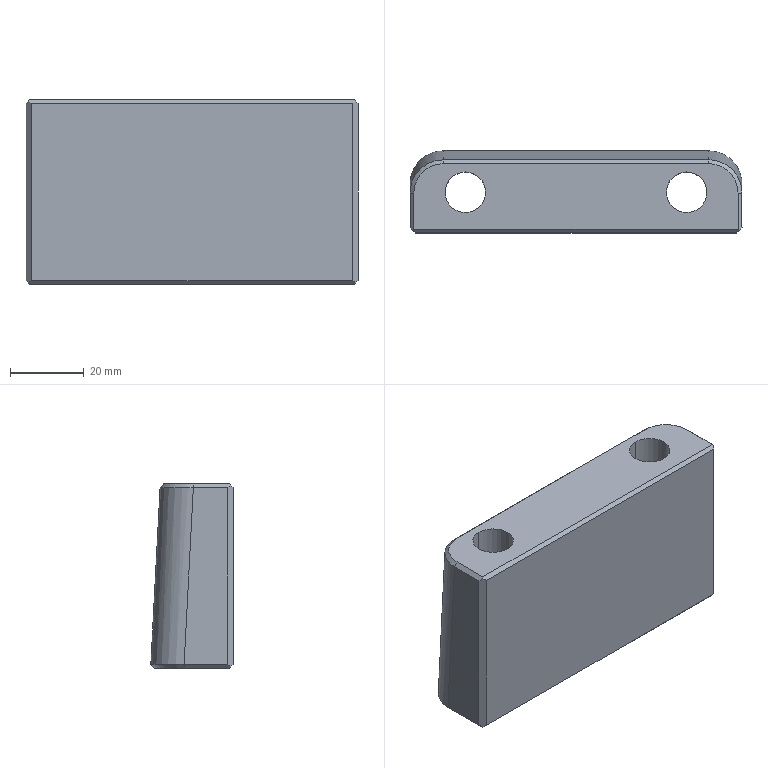Part | Creo | 1 solid | 39 faces | box 90 x 22.317 x 50 mm | volume 78698 mm3 | plane 19 | cylinder 14 | spline 4 | cone 2 | commonest cylinder face diameters 18 x6 11 x4 7 x2 8 x2
STEP:
#1=CARTESIAN_POINT('',(-25.,211.995,61.));
#2=VERTEX_POINT('',#1);
#3=CARTESIAN_POINT('',(-25.,229.995,61.));
#4=VERTEX_POINT('',#3);
#5=CARTESIAN_POINT('',(-25.,220.995,61.));
#6=DIRECTION('',(0.,0.,-1.));
#7=DIRECTION('',(0.000000059,-1.,0.));
#8=AXIS2_PLACEMENT_3D('',#5,#6,#7);
#9=CIRCLE('',#8,9.);
#10=EDGE_CURVE('',#2,#4,#9,.T.);
#11=ORIENTED_EDGE('',*,*,#10,.T.);
#12=CARTESIAN_POINT('',(-25.,229.995,50.));
#13=VERTEX_POINT('',#12);
#14=CARTESIAN_POINT('',(-25.,229.995,50.));
#15=DIRECTION('',(0.,0.,1.));
#16=VECTOR('',#15,11.);
#17=LINE('',#14,#16);
#18=EDGE_CURVE('',#13,#4,#17,.T.);
#19=ORIENTED_EDGE('',*,*,#18,.F.);
#20=CARTESIAN_POINT('',(-34.,220.995,50.));
#21=VERTEX_POINT('',#20);
#22=CARTESIAN_POINT('',(-25.,220.995,50.));
#23=DIRECTION('',(0.,0.,1.));
#24=DIRECTION('',(-0.000000059,1.,0.));
#25=AXIS2_PLACEMENT_3D('',#22,#23,#24);
#26=CIRCLE('',#25,9.);
#27=EDGE_CURVE('',#13,#21,#26,.T.);
#28=ORIENTED_EDGE('',*,*,#27,.T.);
#29=CARTESIAN_POINT('',(-25.,211.995,50.));
#30=VERTEX_POINT('',#29);
#31=CARTESIAN_POINT('',(-25.,220.995,50.));
#32=DIRECTION('',(0.,0.,1.));
#33=DIRECTION('',(-1.,0.,0.));
#34=AXIS2_PLACEMENT_3D('',#31,#32,#33);
#35=CIRCLE('',#34,9.);
#36=EDGE_CURVE('',#21,#30,#35,.T.);
#37=ORIENTED_EDGE('',*,*,#36,.T.);
#38=CARTESIAN_POINT('',(-25.,211.995,50.));
#39=DIRECTION('',(0.,0.,1.));
#40=VECTOR('',#39,11.);
#41=LINE('',#38,#40);
#42=EDGE_CURVE('',#30,#2,#41,.T.);
#43=ORIENTED_EDGE('',*,*,#42,.T.);
#44=EDGE_LOOP('',(#11,#19,#28,#37,#43));
#45=FACE_OUTER_BOUND('',#44,.F.);
#46=CARTESIAN_POINT('',(-25.,220.995,63.45));
#47=DIRECTION('',(0.,0.,1.));
#48=DIRECTION('',(-0.000000059,1.,0.));
#49=AXIS2_PLACEMENT_3D('',#46,#47,#48);
#50=CYLINDRICAL_SURFACE('',#49,9.);
#51=ADVANCED_FACE('',(#45),#50,.F.);
#52=CARTESIAN_POINT('',(-16.,220.995,61.));
#53=VERTEX_POINT('',#52);
#54=CARTESIAN_POINT('',(-25.,220.995,61.));
#55=DIRECTION('',(0.,0.,-1.));
#56=DIRECTION('',(1.,0.,0.));
#57=AXIS2_PLACEMENT_3D('',#54,#55,#56);
#58=CIRCLE('',#57,9.);
#59=EDGE_CURVE('',#53,#2,#58,.T.);
#60=ORIENTED_EDGE('',*,*,#59,.F.);
#61=CARTESIAN_POINT('',(-25.,220.995,61.));
#62=DIRECTION('',(0.,0.,-1.));
#63=DIRECTION('',(-0.000000059,1.,0.));
#64=AXIS2_PLACEMENT_3D('',#61,#62,#63);
#65=CIRCLE('',#64,9.);
#66=EDGE_CURVE('',#4,#53,#65,.T.);
#67=ORIENTED_EDGE('',*,*,#66,.F.);
#68=ORIENTED_EDGE('',*,*,#10,.F.);
#69=EDGE_LOOP('',(#60,#67,#68));
#70=FACE_OUTER_BOUND('',#69,.F.);
#71=CARTESIAN_POINT('',(-19.5,220.995,61.));
#72=VERTEX_POINT('',#71);
#73=CARTESIAN_POINT('',(-25.,226.495,61.));
#74=VERTEX_POINT('',#73);
#75=CARTESIAN_POINT('',(-25.,220.995,61.));
#76=DIRECTION('',(0.,0.,1.));
#77=DIRECTION('',(1.,0.,0.));
#78=AXIS2_PLACEMENT_3D('',#75,#76,#77);
#79=CIRCLE('',#78,5.5);
#80=EDGE_CURVE('',#72,#74,#79,.T.);
#81=ORIENTED_EDGE('',*,*,#80,.F.);
#82=CARTESIAN_POINT('',(-25.,215.495,61.));
#83=VERTEX_POINT('',#82);
#84=CARTESIAN_POINT('',(-25.,220.995,61.));
#85=DIRECTION('',(0.,0.,1.));
#86=DIRECTION('',(0.000000059,-1.,0.));
#87=AXIS2_PLACEMENT_3D('',#84,#85,#86);
#88=CIRCLE('',#87,5.5);
#89=EDGE_CURVE('',#83,#72,#88,.T.);
#90=ORIENTED_EDGE('',*,*,#89,.F.);
#91=CARTESIAN_POINT('',(-25.,220.995,61.));
#92=DIRECTION('',(0.,0.,1.));
#93=DIRECTION('',(-0.000000059,1.,0.));
#94=AXIS2_PLACEMENT_3D('',#91,#92,#93);
#95=CIRCLE('',#94,5.5);
#96=EDGE_CURVE('',#74,#83,#95,.T.);
#97=ORIENTED_EDGE('',*,*,#96,.F.);
#98=EDGE_LOOP('',(#81,#90,#97));
#99=FACE_BOUND('',#98,.F.);
#100=CARTESIAN_POINT('',(-25.,220.995,61.));
#101=DIRECTION('',(0.,0.,1.));
#102=DIRECTION('',(-0.000000059,1.,0.));
#103=AXIS2_PLACEMENT_3D('',#100,#101,#102);
#104=PLANE('',#103);
#105=ADVANCED_FACE('',(#70,#99),#104,.F.);
#106=CARTESIAN_POINT('',(-25.,226.495,100.));
#107=VERTEX_POINT('',#106);
#108=CARTESIAN_POINT('',(-25.,215.495,100.));
#109=VERTEX_POINT('',#108);
#110=CARTESIAN_POINT('',(-25.,220.995,100.));
#111=DIRECTION('',(0.,0.,-1.));
#112=DIRECTION('',(-0.000000059,1.,0.));
#113=AXIS2_PLACEMENT_3D('',#110,#111,#112);
#114=CIRCLE('',#113,5.5);
#115=EDGE_CURVE('',#107,#109,#114,.T.);
#116=ORIENTED_EDGE('',*,*,#115,.T.);
#117=CARTESIAN_POINT('',(-25.,215.495,100.));
#118=DIRECTION('',(0.,0.,-1.));
#119=VECTOR('',#118,39.);
#120=LINE('',#117,#119);
#121=EDGE_CURVE('',#109,#83,#120,.T.);
#122=ORIENTED_EDGE('',*,*,#121,.T.);
#123=ORIENTED_EDGE('',*,*,#89,.T.);
#124=ORIENTED_EDGE('',*,*,#80,.T.);
#125=CARTESIAN_POINT('',(-25.,226.495,100.));
#126=DIRECTION('',(0.,0.,-1.));
#127=VECTOR('',#126,39.);
#128=LINE('',#125,#127);
#129=EDGE_CURVE('',#107,#74,#128,.T.);
#130=ORIENTED_EDGE('',*,*,#129,.F.);
#131=EDGE_LOOP('',(#116,#122,#123,#124,#130));
#132=FACE_OUTER_BOUND('',#131,.F.);
#133=CARTESIAN_POINT('',(-25.,220.995,75.));
#134=DIRECTION('',(0.,0.,-1.));
#135=DIRECTION('',(-0.000000059,1.,0.));
#136=AXIS2_PLACEMENT_3D('',#133,#134,#135);
#137=CYLINDRICAL_SURFACE('',#136,5.5);
#138=ADVANCED_FACE('',(#132),#137,.F.);
#139=CARTESIAN_POINT('',(-91.,228.755,100.));
#140=VERTEX_POINT('',#139);
#141=CARTESIAN_POINT('',(-98.946,220.797,100.));
#142=VERTEX_POINT('',#141);
#143=CARTESIAN_POINT('',(-93.083,228.763,100.));
#144=CARTESIAN_POINT('',(-97.219,227.025,100.));
#145=CARTESIAN_POINT('',(-98.955,222.883,100.));
#146=B_SPLINE_CURVE_WITH_KNOTS('',3,(#139,#143,#144,#145,#141),.UNSPECIFIED.,.F.,.F.,(4,1,4),(0.,0.5,1.),.UNSPECIFIED.);
#147=EDGE_CURVE('',#140,#142,#146,.T.);
#148=ORIENTED_EDGE('',*,*,#147,.F.);
#149=CARTESIAN_POINT('',(-19.,228.755,100.));
#150=VERTEX_POINT('',#149);
#151=CARTESIAN_POINT('',(-91.,228.755,100.));
#152=DIRECTION('',(1.,0.000000059,0.));
#153=VECTOR('',#152,72.);
#154=LINE('',#151,#153);
#155=EDGE_CURVE('',#140,#150,#154,.T.);
#156=ORIENTED_EDGE('',*,*,#155,.T.);
#157=CARTESIAN_POINT('',(-11.054,220.797,100.));
#158=VERTEX_POINT('',#157);
#159=CARTESIAN_POINT('',(-11.054,220.797,100.));
#160=CARTESIAN_POINT('',(-11.045,222.883,100.));
#161=CARTESIAN_POINT('',(-12.781,227.025,100.));
#162=CARTESIAN_POINT('',(-16.917,228.763,100.));
#163=B_SPLINE_CURVE_WITH_KNOTS('',3,(#159,#160,#161,#162,#149),.UNSPECIFIED.,.F.,.F.,(4,1,4),(0.,0.5,1.),.UNSPECIFIED.);
#164=EDGE_CURVE('',#158,#150,#163,.T.);
#165=ORIENTED_EDGE('',*,*,#164,.F.);
#166=CARTESIAN_POINT('',(-11.054,210.944,100.));
#167=VERTEX_POINT('',#166);
#168=CARTESIAN_POINT('',(-11.054,220.797,100.));
#169=DIRECTION('',(0.000000059,-1.,0.));
#170=VECTOR('',#169,9.853);
#171=LINE('',#168,#170);
#172=EDGE_CURVE('',#158,#167,#171,.T.);
#173=ORIENTED_EDGE('',*,*,#172,.T.);
#174=CARTESIAN_POINT('',(-98.946,210.944,100.));
#175=VERTEX_POINT('',#174);
#176=CARTESIAN_POINT('',(-11.054,210.944,100.));
#177=DIRECTION('',(-1.,-0.000000059,0.));
#178=VECTOR('',#177,87.892);
#179=LINE('',#176,#178);
#180=EDGE_CURVE('',#167,#175,#179,.T.);
#181=ORIENTED_EDGE('',*,*,#180,.T.);
#182=CARTESIAN_POINT('',(-98.946,210.944,100.));
#183=DIRECTION('',(-0.000000059,1.,0.));
#184=VECTOR('',#183,9.853);
#185=LINE('',#182,#184);
#186=EDGE_CURVE('',#175,#142,#185,.T.);
#187=ORIENTED_EDGE('',*,*,#186,.T.);
#188=EDGE_LOOP('',(#148,#156,#165,#173,#181,#187));
#189=FACE_OUTER_BOUND('',#188,.F.);
#190=ORIENTED_EDGE('',*,*,#115,.F.);
#191=CARTESIAN_POINT('',(-25.,220.995,100.));
#192=DIRECTION('',(0.,0.,-1.));
#193=DIRECTION('',(0.000000059,-1.,0.));
#194=AXIS2_PLACEMENT_3D('',#191,#192,#193);
#195=CIRCLE('',#194,5.5);
#196=EDGE_CURVE('',#109,#107,#195,.T.);
#197=ORIENTED_EDGE('',*,*,#196,.F.);
#198=EDGE_LOOP('',(#190,#197));
#199=FACE_BOUND('',#198,.F.);
#200=CARTESIAN_POINT('',(-85.,226.495,100.));
#201=VERTEX_POINT('',#200);
#202=CARTESIAN_POINT('',(-85.,215.495,100.));
#203=VERTEX_POINT('',#202);
#204=CARTESIAN_POINT('',(-85.,220.995,100.));
#205=DIRECTION('',(0.,0.,-1.));
#206=DIRECTION('',(-0.000000059,1.,0.));
#207=AXIS2_PLACEMENT_3D('',#204,#205,#206);
#208=CIRCLE('',#207,5.5);
#209=EDGE_CURVE('',#201,#203,#208,.T.);
#210=ORIENTED_EDGE('',*,*,#209,.F.);
#211=CARTESIAN_POINT('',(-85.,220.995,100.));
#212=DIRECTION('',(0.,0.,-1.));
#213=DIRECTION('',(0.000000059,-1.,0.));
#214=AXIS2_PLACEMENT_3D('',#211,#212,#213);
#215=CIRCLE('',#214,5.5);
#216=EDGE_CURVE('',#203,#201,#215,.T.);
#217=ORIENTED_EDGE('',*,*,#216,.F.);
#218=EDGE_LOOP('',(#210,#217));
#219=FACE_BOUND('',#218,.F.);
#220=CARTESIAN_POINT('',(-10.,209.995,100.));
#221=DIRECTION('',(0.,0.,1.));
#222=DIRECTION('',(-0.000000059,1.,0.));
#223=AXIS2_PLACEMENT_3D('',#220,#221,#222);
#224=PLANE('',#223);
#225=ADVANCED_FACE('',(#189,#199,#219),#224,.T.);
#226=CARTESIAN_POINT('',(-91.,229.807,99.001));
#227=VERTEX_POINT('',#226);
#228=CARTESIAN_POINT('',(-91.,228.755,100.));
#229=DIRECTION('',(0.000000048,0.7254,-0.6884));
#230=VECTOR('',#229,1.451);
#231=LINE('',#228,#230);
#232=EDGE_CURVE('',#140,#227,#231,.T.);
#233=ORIENTED_EDGE('',*,*,#232,.F.);
#234=ORIENTED_EDGE('',*,*,#147,.T.);
#235=CARTESIAN_POINT('',(-100.,220.797,98.946));
#236=VERTEX_POINT('',#235);
#237=CARTESIAN_POINT('',(-100.,220.797,98.946));
#238=DIRECTION('',(0.7071,0.000000042,0.7071));
#239=VECTOR('',#238,1.49);
#240=LINE('',#237,#239);
#241=EDGE_CURVE('',#236,#142,#240,.T.);
#242=ORIENTED_EDGE('',*,*,#241,.F.);
#243=CARTESIAN_POINT('',(-91.,229.807,99.001));
#244=CARTESIAN_POINT('',(-91.278,229.807,99.003));
#245=CARTESIAN_POINT('',(-91.835,229.781,99.003));
#246=CARTESIAN_POINT('',(-92.662,229.665,99.));
#247=CARTESIAN_POINT('',(-93.474,229.473,98.996));
#248=CARTESIAN_POINT('',(-94.266,229.207,98.992));
#249=CARTESIAN_POINT('',(-95.03,228.868,98.989));
#250=CARTESIAN_POINT('',(-95.758,228.46,98.988));
#251=CARTESIAN_POINT('',(-96.441,227.99,98.988));
#252=CARTESIAN_POINT('',(-97.075,227.462,98.987));
#253=CARTESIAN_POINT('',(-97.656,226.881,98.984));
#254=CARTESIAN_POINT('',(-98.183,226.246,98.977));
#255=CARTESIAN_POINT('',(-98.654,225.562,98.97));
#256=CARTESIAN_POINT('',(-99.061,224.834,98.965));
#257=CARTESIAN_POINT('',(-99.4,224.068,98.96));
#258=CARTESIAN_POINT('',(-99.667,223.275,98.958));
#259=CARTESIAN_POINT('',(-99.858,222.461,98.956));
#260=CARTESIAN_POINT('',(-99.974,221.632,98.953));
#261=CARTESIAN_POINT('',(-100.,221.076,98.949));
#262=CARTESIAN_POINT('',(-100.,220.797,98.946));
#263=B_SPLINE_CURVE_WITH_KNOTS('',3,(#243,#244,#245,#246,#247,#248,#249,#250,#251,#252,#253,#254,#255,#256,#257,#258,#259,#260,#261,#262),.UNSPECIFIED.,.F.,.F.,(4,1,1,1,1,1,1,1,1,1,1,1,1,1,1,1,1,4),(0.,0.05882,0.1176,0.1765,0.2353,0.2941,0.3529,0.4118,0.4706,0.5294,0.5882,0.6471,0.7059,0.7647,0.8235,0.8824,0.9412,1.),.UNSPECIFIED.);
#264=EDGE_CURVE('',#227,#236,#263,.T.);
#265=ORIENTED_EDGE('',*,*,#264,.F.);
#266=EDGE_LOOP('',(#233,#234,#242,#265));
#267=FACE_OUTER_BOUND('',#266,.F.);
#268=CARTESIAN_POINT('',(-90.877,228.661,100.087));
#269=CARTESIAN_POINT('',(-90.87,229.075,99.694));
#270=CARTESIAN_POINT('',(-90.864,229.489,99.301));
#271=CARTESIAN_POINT('',(-90.857,229.903,98.908));
#272=CARTESIAN_POINT('',(-90.918,228.662,100.087));
#273=CARTESIAN_POINT('',(-90.913,229.076,99.694));
#274=CARTESIAN_POINT('',(-90.909,229.49,99.301));
#275=CARTESIAN_POINT('',(-90.905,229.904,98.908));
#276=CARTESIAN_POINT('',(-93.018,228.688,100.087));
#277=CARTESIAN_POINT('',(-93.125,229.104,99.694));
#278=CARTESIAN_POINT('',(-93.231,229.519,99.301));
#279=CARTESIAN_POINT('',(-93.338,229.935,98.908));
#280=CARTESIAN_POINT('',(-97.147,226.953,100.088));
#281=CARTESIAN_POINT('',(-97.471,227.277,99.691));
#282=CARTESIAN_POINT('',(-97.796,227.601,99.293));
#283=CARTESIAN_POINT('',(-98.12,227.925,98.895));
#284=CARTESIAN_POINT('',(-98.88,222.819,100.091));
#285=CARTESIAN_POINT('',(-99.296,222.925,99.682));
#286=CARTESIAN_POINT('',(-99.712,223.031,99.272));
#287=CARTESIAN_POINT('',(-100.128,223.138,98.863));
#288=CARTESIAN_POINT('',(-98.853,220.715,100.092));
#289=CARTESIAN_POINT('',(-99.268,220.711,99.677));
#290=CARTESIAN_POINT('',(-99.683,220.706,99.262));
#291=CARTESIAN_POINT('',(-100.098,220.702,98.847));
#292=CARTESIAN_POINT('',(-98.853,220.674,100.092));
#293=CARTESIAN_POINT('',(-99.267,220.667,99.677));
#294=CARTESIAN_POINT('',(-99.682,220.661,99.262));
#295=CARTESIAN_POINT('',(-100.097,220.654,98.847));
#296=B_SPLINE_SURFACE_WITH_KNOTS('',3,3,((#268,#269,#270,#271),(#272,#273,#274,#275),(#276,#277,#278,#279),(#280,#281,#282,#283),(#284,#285,#286,#287),(#288,#289,#290,#291),(#292,#293,#294,#295)),.UNSPECIFIED.,.F.,.F.,.F.,(4,1,1,1,4),(4,4),(-0.009987,0.,0.5,1.,1.01),(-0.08638,1.081),.UNSPECIFIED.);
#297=ADVANCED_FACE('',(#267),#296,.F.);
#298=CARTESIAN_POINT('',(-19.,229.807,99.001));
#299=VERTEX_POINT('',#298);
#300=CARTESIAN_POINT('',(-19.,229.807,99.001));
#301=DIRECTION('',(-0.000000048,-0.7254,0.6884));
#302=VECTOR('',#301,1.451);
#303=LINE('',#300,#302);
#304=EDGE_CURVE('',#299,#150,#303,.T.);
#305=ORIENTED_EDGE('',*,*,#304,.T.);
#306=ORIENTED_EDGE('',*,*,#155,.F.);
#307=ORIENTED_EDGE('',*,*,#232,.T.);
#308=CARTESIAN_POINT('',(-19.,229.807,99.001));
#309=DIRECTION('',(-1.,-0.000000059,0.));
#310=VECTOR('',#309,72.);
#311=LINE('',#308,#310);
#312=EDGE_CURVE('',#299,#227,#311,.T.);
#313=ORIENTED_EDGE('',*,*,#312,.F.);
#314=EDGE_LOOP('',(#305,#306,#307,#313));
#315=FACE_OUTER_BOUND('',#314,.F.);
#316=CARTESIAN_POINT('',(-10.,229.807,99.001));
#317=DIRECTION('',(0.00000004,-0.6884,-0.7254));
#318=DIRECTION('',(1.,0.000000059,0.));
#319=AXIS2_PLACEMENT_3D('',#316,#317,#318);
#320=PLANE('',#319);
#321=ADVANCED_FACE('',(#315),#320,.F.);
#322=CARTESIAN_POINT('',(-10.,220.797,98.946));
#323=VERTEX_POINT('',#322);
#324=CARTESIAN_POINT('',(-11.054,220.797,100.));
#325=DIRECTION('',(0.7071,0.000000041,-0.7071));
#326=VECTOR('',#325,1.49);
#327=LINE('',#324,#326);
#328=EDGE_CURVE('',#158,#323,#327,.T.);
#329=ORIENTED_EDGE('',*,*,#328,.F.);
#330=ORIENTED_EDGE('',*,*,#164,.T.);
#331=ORIENTED_EDGE('',*,*,#304,.F.);
#332=CARTESIAN_POINT('',(-10.,220.797,98.946));
#333=CARTESIAN_POINT('',(-10.,221.076,98.949));
#334=CARTESIAN_POINT('',(-10.026,221.632,98.953));
#335=CARTESIAN_POINT('',(-10.142,222.461,98.956));
#336=CARTESIAN_POINT('',(-10.333,223.275,98.958));
#337=CARTESIAN_POINT('',(-10.6,224.068,98.96));
#338=CARTESIAN_POINT('',(-10.939,224.834,98.965));
#339=CARTESIAN_POINT('',(-11.346,225.562,98.97));
#340=CARTESIAN_POINT('',(-11.817,226.247,98.977));
#341=CARTESIAN_POINT('',(-12.345,226.881,98.984));
#342=CARTESIAN_POINT('',(-12.926,227.462,98.987));
#343=CARTESIAN_POINT('',(-13.559,227.99,98.988));
#344=CARTESIAN_POINT('',(-14.242,228.461,98.988));
#345=CARTESIAN_POINT('',(-14.97,228.868,98.989));
#346=CARTESIAN_POINT('',(-15.734,229.207,98.992));
#347=CARTESIAN_POINT('',(-16.526,229.473,98.996));
#348=CARTESIAN_POINT('',(-17.338,229.665,99.));
#349=CARTESIAN_POINT('',(-18.165,229.781,99.003));
#350=CARTESIAN_POINT('',(-18.722,229.807,99.003));
#351=CARTESIAN_POINT('',(-19.,229.807,99.001));
#352=B_SPLINE_CURVE_WITH_KNOTS('',3,(#332,#333,#334,#335,#336,#337,#338,#339,#340,#341,#342,#343,#344,#345,#346,#347,#348,#349,#350,#351),.UNSPECIFIED.,.F.,.F.,(4,1,1,1,1,1,1,1,1,1,1,1,1,1,1,1,1,4),(0.,0.05882,0.1176,0.1765,0.2353,0.2941,0.3529,0.4118,0.4706,0.5294,0.5882,0.6471,0.7059,0.7647,0.8235,0.8824,0.9412,1.),.UNSPECIFIED.);
#353=EDGE_CURVE('',#323,#299,#352,.T.);
#354=ORIENTED_EDGE('',*,*,#353,.F.);
#355=EDGE_LOOP('',(#329,#330,#331,#354));
#356=FACE_OUTER_BOUND('',#355,.F.);
#357=CARTESIAN_POINT('',(-11.147,220.674,100.092));
#358=CARTESIAN_POINT('',(-10.733,220.667,99.677));
#359=CARTESIAN_POINT('',(-10.318,220.661,99.262));
#360=CARTESIAN_POINT('',(-9.903,220.654,98.847));
#361=CARTESIAN_POINT('',(-11.147,220.715,100.092));
#362=CARTESIAN_POINT('',(-10.732,220.711,99.677));
#363=CARTESIAN_POINT('',(-10.317,220.706,99.262));
#364=CARTESIAN_POINT('',(-9.902,220.702,98.847));
#365=CARTESIAN_POINT('',(-11.12,222.819,100.091));
#366=CARTESIAN_POINT('',(-10.704,222.925,99.682));
#367=CARTESIAN_POINT('',(-10.288,223.031,99.272));
#368=CARTESIAN_POINT('',(-9.872,223.138,98.863));
#369=CARTESIAN_POINT('',(-12.853,226.953,100.088));
#370=CARTESIAN_POINT('',(-12.529,227.277,99.691));
#371=CARTESIAN_POINT('',(-12.204,227.601,99.293));
#372=CARTESIAN_POINT('',(-11.88,227.925,98.895));
#373=CARTESIAN_POINT('',(-16.982,228.688,100.087));
#374=CARTESIAN_POINT('',(-16.875,229.104,99.694));
#375=CARTESIAN_POINT('',(-16.769,229.519,99.301));
#376=CARTESIAN_POINT('',(-16.662,229.935,98.908));
#377=CARTESIAN_POINT('',(-19.082,228.662,100.087));
#378=CARTESIAN_POINT('',(-19.087,229.076,99.694));
#379=CARTESIAN_POINT('',(-19.091,229.49,99.301));
#380=CARTESIAN_POINT('',(-19.095,229.904,98.908));
#381=CARTESIAN_POINT('',(-19.123,228.661,100.087));
#382=CARTESIAN_POINT('',(-19.13,229.075,99.694));
#383=CARTESIAN_POINT('',(-19.136,229.489,99.301));
#384=CARTESIAN_POINT('',(-19.143,229.903,98.908));
#385=B_SPLINE_SURFACE_WITH_KNOTS('',3,3,((#357,#358,#359,#360),(#361,#362,#363,#364),(#365,#366,#367,#368),(#369,#370,#371,#372),(#373,#374,#375,#376),(#377,#378,#379,#380),(#381,#382,#383,#384)),.UNSPECIFIED.,.F.,.F.,.F.,(4,1,1,1,4),(4,4),(-0.009975,0.,0.5,1.,1.01),(-0.08638,1.081),.UNSPECIFIED.);
#386=ADVANCED_FACE('',(#356),#385,.F.);
#387=CARTESIAN_POINT('',(-10.764,210.655,99.71));
#388=VERTEX_POINT('',#387);
#389=CARTESIAN_POINT('',(-10.,211.419,98.946));
#390=VERTEX_POINT('',#389);
#391=CARTESIAN_POINT('',(-10.764,210.655,99.71));
#392=DIRECTION('',(0.5774,0.5774,-0.5774));
#393=VECTOR('',#392,1.324);
#394=LINE('',#391,#393);
#395=EDGE_CURVE('',#388,#390,#394,.T.);
#396=ORIENTED_EDGE('',*,*,#395,.F.);
#397=CARTESIAN_POINT('',(-11.054,210.944,100.));
#398=DIRECTION('',(0.5774,-0.5774,-0.5774));
#399=VECTOR('',#398,0.5017);
#400=LINE('',#397,#399);
#401=EDGE_CURVE('',#167,#388,#400,.T.);
#402=ORIENTED_EDGE('',*,*,#401,.F.);
#403=ORIENTED_EDGE('',*,*,#172,.F.);
#404=ORIENTED_EDGE('',*,*,#328,.T.);
#405=CARTESIAN_POINT('',(-10.,211.419,98.946));
#406=DIRECTION('',(-0.000000059,1.,0.));
#407=VECTOR('',#406,9.379);
#408=LINE('',#405,#407);
#409=EDGE_CURVE('',#390,#323,#408,.T.);
#410=ORIENTED_EDGE('',*,*,#409,.F.);
#411=EDGE_LOOP('',(#396,#402,#403,#404,#410));
#412=FACE_OUTER_BOUND('',#411,.F.);
#413=CARTESIAN_POINT('',(-10.,209.995,98.946));
#414=DIRECTION('',(0.7071,0.000000042,0.7071));
#415=DIRECTION('',(-0.000000059,1.,0.));
#416=AXIS2_PLACEMENT_3D('',#413,#414,#415);
#417=PLANE('',#416);
#418=ADVANCED_FACE('',(#412),#417,.T.);
#419=CARTESIAN_POINT('',(-10.739,210.68,50.315));
#420=VERTEX_POINT('',#419);
#421=CARTESIAN_POINT('',(-11.419,210.,50.995));
#422=VERTEX_POINT('',#421);
#423=CARTESIAN_POINT('',(-10.739,210.68,50.315));
#424=DIRECTION('',(-0.5774,-0.5774,0.5774));
#425=VECTOR('',#424,1.178);
#426=LINE('',#423,#425);
#427=EDGE_CURVE('',#420,#422,#426,.T.);
#428=ORIENTED_EDGE('',*,*,#427,.T.);
#429=CARTESIAN_POINT('',(-11.419,210.,99.056));
#430=VERTEX_POINT('',#429);
#431=CARTESIAN_POINT('',(-11.419,210.,50.995));
#432=DIRECTION('',(0.,0.,1.));
#433=VECTOR('',#432,48.06);
#434=LINE('',#431,#433);
#435=EDGE_CURVE('',#422,#430,#434,.T.);
#436=ORIENTED_EDGE('',*,*,#435,.T.);
#437=CARTESIAN_POINT('',(-11.419,210.,99.056));
#438=DIRECTION('',(0.5774,0.5774,0.5774));
#439=VECTOR('',#438,1.134);
#440=LINE('',#437,#439);
#441=EDGE_CURVE('',#430,#388,#440,.T.);
#442=ORIENTED_EDGE('',*,*,#441,.T.);
#443=ORIENTED_EDGE('',*,*,#395,.T.);
#444=CARTESIAN_POINT('',(-10.,211.419,51.054));
#445=VERTEX_POINT('',#444);
#446=CARTESIAN_POINT('',(-10.,211.419,51.054));
#447=DIRECTION('',(0.,0.,1.));
#448=VECTOR('',#447,47.892);
#449=LINE('',#446,#448);
#450=EDGE_CURVE('',#445,#390,#449,.T.);
#451=ORIENTED_EDGE('',*,*,#450,.F.);
#452=CARTESIAN_POINT('',(-10.,211.419,51.054));
#453=DIRECTION('',(-0.5774,-0.5774,-0.5774));
#454=VECTOR('',#453,1.279);
#455=LINE('',#452,#454);
#456=EDGE_CURVE('',#445,#420,#455,.T.);
#457=ORIENTED_EDGE('',*,*,#456,.T.);
#458=EDGE_LOOP('',(#428,#436,#442,#443,#451,#457));
#459=FACE_OUTER_BOUND('',#458,.F.);
#460=CARTESIAN_POINT('',(-10.712,210.707,49.21));
#461=DIRECTION('',(0.7071,-0.7071,0.));
#462=DIRECTION('',(-0.7071,-0.7071,0.));
#463=AXIS2_PLACEMENT_3D('',#460,#461,#462);
#464=PLANE('',#463);
#465=ADVANCED_FACE('',(#459),#464,.T.);
#466=CARTESIAN_POINT('',(-44.912,210.,50.995));
#467=VERTEX_POINT('',#466);
#468=CARTESIAN_POINT('',(-11.419,210.,50.995));
#469=DIRECTION('',(-1.,-0.000000059,0.));
#470=VECTOR('',#469,33.494);
#471=LINE('',#468,#470);
#472=EDGE_CURVE('',#422,#467,#471,.T.);
#473=ORIENTED_EDGE('',*,*,#472,.F.);
#474=ORIENTED_EDGE('',*,*,#427,.F.);
#475=CARTESIAN_POINT('',(-11.054,210.995,50.));
#476=VERTEX_POINT('',#475);
#477=CARTESIAN_POINT('',(-10.739,210.68,50.315));
#478=DIRECTION('',(-0.5774,0.5774,-0.5774));
#479=VECTOR('',#478,0.5459);
#480=LINE('',#477,#479);
#481=EDGE_CURVE('',#420,#476,#480,.T.);
#482=ORIENTED_EDGE('',*,*,#481,.T.);
#483=CARTESIAN_POINT('',(-98.946,210.995,50.));
#484=VERTEX_POINT('',#483);
#485=CARTESIAN_POINT('',(-98.946,210.995,50.));
#486=DIRECTION('',(1.,0.000000059,0.));
#487=VECTOR('',#486,87.892);
#488=LINE('',#485,#487);
#489=EDGE_CURVE('',#484,#476,#488,.T.);
#490=ORIENTED_EDGE('',*,*,#489,.F.);
#491=CARTESIAN_POINT('',(-99.261,210.68,50.315));
#492=VERTEX_POINT('',#491);
#493=CARTESIAN_POINT('',(-98.946,210.995,50.));
#494=DIRECTION('',(-0.5774,-0.5774,0.5774));
#495=VECTOR('',#494,0.5459);
#496=LINE('',#493,#495);
#497=EDGE_CURVE('',#484,#492,#496,.T.);
#498=ORIENTED_EDGE('',*,*,#497,.T.);
#499=CARTESIAN_POINT('',(-98.581,210.,50.995));
#500=VERTEX_POINT('',#499);
#501=CARTESIAN_POINT('',(-98.581,210.,50.995));
#502=DIRECTION('',(-0.5774,0.5774,-0.5774));
#503=VECTOR('',#502,1.178);
#504=LINE('',#501,#503);
#505=EDGE_CURVE('',#500,#492,#504,.T.);
#506=ORIENTED_EDGE('',*,*,#505,.F.);
#507=CARTESIAN_POINT('',(-53.088,210.,50.995));
#508=VERTEX_POINT('',#507);
#509=CARTESIAN_POINT('',(-53.088,210.,50.995));
#510=DIRECTION('',(-1.,-0.000000059,0.));
#511=VECTOR('',#510,45.494);
#512=LINE('',#509,#511);
#513=EDGE_CURVE('',#508,#500,#512,.T.);
#514=ORIENTED_EDGE('',*,*,#513,.F.);
#515=CARTESIAN_POINT('',(-44.912,210.,50.995));
#516=DIRECTION('',(-1.,-0.000000059,0.));
#517=VECTOR('',#516,8.175);
#518=LINE('',#515,#517);
#519=EDGE_CURVE('',#467,#508,#518,.T.);
#520=ORIENTED_EDGE('',*,*,#519,.F.);
#521=EDGE_LOOP('',(#473,#474,#482,#490,#498,#506,#514,#520));
#522=FACE_OUTER_BOUND('',#521,.F.);
#523=CARTESIAN_POINT('',(-10.,209.995,51.));
#524=DIRECTION('',(-0.000000042,0.7071,0.7071));
#525=DIRECTION('',(1.,0.000000059,0.));
#526=AXIS2_PLACEMENT_3D('',#523,#524,#525);
#527=PLANE('',#526);
#528=ADVANCED_FACE('',(#522),#527,.F.);
#529=ORIENTED_EDGE('',*,*,#519,.T.);
#530=ORIENTED_EDGE('',*,*,#513,.T.);
#531=CARTESIAN_POINT('',(-98.581,210.,99.056));
#532=VERTEX_POINT('',#531);
#533=CARTESIAN_POINT('',(-98.581,210.,99.056));
#534=DIRECTION('',(0.,0.,-1.));
#535=VECTOR('',#534,48.06);
#536=LINE('',#533,#535);
#537=EDGE_CURVE('',#532,#500,#536,.T.);
#538=ORIENTED_EDGE('',*,*,#537,.F.);
#539=CARTESIAN_POINT('',(-11.419,210.,99.056));
#540=DIRECTION('',(-1.,-0.000000059,0.));
#541=VECTOR('',#540,87.162);
#542=LINE('',#539,#541);
#543=EDGE_CURVE('',#430,#532,#542,.T.);
#544=ORIENTED_EDGE('',*,*,#543,.F.);
#545=ORIENTED_EDGE('',*,*,#435,.F.);
#546=ORIENTED_EDGE('',*,*,#472,.T.);
#547=EDGE_LOOP('',(#529,#530,#538,#544,#545,#546));
#548=FACE_OUTER_BOUND('',#547,.F.);
#549=CARTESIAN_POINT('',(-10.,210.,0.));
#550=DIRECTION('',(0.000000059,-1.,0.));
#551=DIRECTION('',(0.,0.,1.));
#552=AXIS2_PLACEMENT_3D('',#549,#550,#551);
#553=PLANE('',#552);
#554=ADVANCED_FACE('',(#548),#553,.T.);
#555=CARTESIAN_POINT('',(-100.,211.419,98.946));
#556=VERTEX_POINT('',#555);
#557=CARTESIAN_POINT('',(-100.,211.419,51.054));
#558=VERTEX_POINT('',#557);
#559=CARTESIAN_POINT('',(-100.,211.419,98.946));
#560=DIRECTION('',(0.,0.,-1.));
#561=VECTOR('',#560,47.892);
#562=LINE('',#559,#561);
#563=EDGE_CURVE('',#556,#558,#562,.T.);
#564=ORIENTED_EDGE('',*,*,#563,.F.);
#565=CARTESIAN_POINT('',(-99.236,210.655,99.71));
#566=VERTEX_POINT('',#565);
#567=CARTESIAN_POINT('',(-100.,211.419,98.946));
#568=DIRECTION('',(0.5774,-0.5774,0.5774));
#569=VECTOR('',#568,1.324);
#570=LINE('',#567,#569);
#571=EDGE_CURVE('',#556,#566,#570,.T.);
#572=ORIENTED_EDGE('',*,*,#571,.T.);
#573=CARTESIAN_POINT('',(-99.236,210.655,99.71));
#574=DIRECTION('',(0.5774,-0.5774,-0.5774));
#575=VECTOR('',#574,1.134);
#576=LINE('',#573,#575);
#577=EDGE_CURVE('',#566,#532,#576,.T.);
#578=ORIENTED_EDGE('',*,*,#577,.T.);
#579=ORIENTED_EDGE('',*,*,#537,.T.);
#580=ORIENTED_EDGE('',*,*,#505,.T.);
#581=CARTESIAN_POINT('',(-99.261,210.68,50.315));
#582=DIRECTION('',(-0.5774,0.5774,0.5774));
#583=VECTOR('',#582,1.279);
#584=LINE('',#581,#583);
#585=EDGE_CURVE('',#492,#558,#584,.T.);
#586=ORIENTED_EDGE('',*,*,#585,.T.);
#587=EDGE_LOOP('',(#564,#572,#578,#579,#580,#586));
#588=FACE_OUTER_BOUND('',#587,.F.);
#589=CARTESIAN_POINT('',(-99.288,210.707,49.21));
#590=DIRECTION('',(-0.7071,-0.7071,0.));
#591=DIRECTION('',(0.7071,-0.7071,0.));
#592=AXIS2_PLACEMENT_3D('',#589,#590,#591);
#593=PLANE('',#592);
#594=ADVANCED_FACE('',(#588),#593,.T.);
#595=CARTESIAN_POINT('',(-100.,223.307,51.054));
#596=VERTEX_POINT('',#595);
#597=CARTESIAN_POINT('',(-100.,220.797,98.946));
#598=DIRECTION('',(-0.000000003,0.05234,-0.9986));
#599=VECTOR('',#598,47.958);
#600=LINE('',#597,#599);
#601=EDGE_CURVE('',#236,#596,#600,.T.);
#602=ORIENTED_EDGE('',*,*,#601,.F.);
#603=CARTESIAN_POINT('',(-100.,220.797,98.946));
#604=DIRECTION('',(0.000000059,-1.,0.));
#605=VECTOR('',#604,9.379);
#606=LINE('',#603,#605);
#607=EDGE_CURVE('',#236,#556,#606,.T.);
#608=ORIENTED_EDGE('',*,*,#607,.T.);
#609=ORIENTED_EDGE('',*,*,#563,.T.);
#610=CARTESIAN_POINT('',(-100.,211.419,51.054));
#611=DIRECTION('',(-0.000000059,1.,0.));
#612=VECTOR('',#611,11.889);
#613=LINE('',#610,#612);
#614=EDGE_CURVE('',#558,#596,#613,.T.);
#615=ORIENTED_EDGE('',*,*,#614,.T.);
#616=EDGE_LOOP('',(#602,#608,#609,#615));
#617=FACE_OUTER_BOUND('',#616,.F.);
#618=CARTESIAN_POINT('',(-100.,209.995,0.));
#619=DIRECTION('',(-1.,-0.000000059,0.));
#620=DIRECTION('',(-0.000000059,1.,0.));
#621=AXIS2_PLACEMENT_3D('',#618,#619,#620);
#622=PLANE('',#621);
#623=ADVANCED_FACE('',(#617),#622,.T.);
#624=CARTESIAN_POINT('',(-91.,232.317,51.109));
#625=VERTEX_POINT('',#624);
#626=CARTESIAN_POINT('',(-91.,229.807,99.001));
#627=DIRECTION('',(-0.000000003,0.05234,-0.9986));
#628=VECTOR('',#627,47.958);
#629=LINE('',#626,#628);
#630=EDGE_CURVE('',#227,#625,#629,.T.);
#631=ORIENTED_EDGE('',*,*,#630,.F.);
#632=ORIENTED_EDGE('',*,*,#264,.T.);
#633=ORIENTED_EDGE('',*,*,#601,.T.);
#634=CARTESIAN_POINT('',(-100.,223.307,51.054));
#635=CARTESIAN_POINT('',(-100.,223.586,51.054));
#636=CARTESIAN_POINT('',(-99.974,224.143,51.057));
#637=CARTESIAN_POINT('',(-99.858,224.972,51.065));
#638=CARTESIAN_POINT('',(-99.666,225.786,51.073));
#639=CARTESIAN_POINT('',(-99.399,226.58,51.08));
#640=CARTESIAN_POINT('',(-99.06,227.345,51.085));
#641=CARTESIAN_POINT('',(-98.652,228.074,51.088));
#642=CARTESIAN_POINT('',(-98.182,228.758,51.09));
#643=CARTESIAN_POINT('',(-97.654,229.393,51.091));
#644=CARTESIAN_POINT('',(-97.073,229.974,51.095));
#645=CARTESIAN_POINT('',(-96.439,230.501,51.1));
#646=CARTESIAN_POINT('',(-95.755,230.972,51.106));
#647=CARTESIAN_POINT('',(-95.027,231.379,51.109));
#648=CARTESIAN_POINT('',(-94.263,231.718,51.111));
#649=CARTESIAN_POINT('',(-93.47,231.984,51.11));
#650=CARTESIAN_POINT('',(-92.658,232.176,51.109));
#651=CARTESIAN_POINT('',(-91.832,232.291,51.107));
#652=CARTESIAN_POINT('',(-91.277,232.317,51.108));
#653=CARTESIAN_POINT('',(-91.,232.317,51.109));
#654=B_SPLINE_CURVE_WITH_KNOTS('',3,(#634,#635,#636,#637,#638,#639,#640,#641,#642,#643,#644,#645,#646,#647,#648,#649,#650,#651,#652,#653),.UNSPECIFIED.,.F.,.F.,(4,1,1,1,1,1,1,1,1,1,1,1,1,1,1,1,1,4),(0.,0.05882,0.1176,0.1765,0.2353,0.2941,0.3529,0.4118,0.4706,0.5294,0.5882,0.6471,0.7059,0.7647,0.8235,0.8824,0.9412,1.),.UNSPECIFIED.);
#655=EDGE_CURVE('',#596,#625,#654,.T.);
#656=ORIENTED_EDGE('',*,*,#655,.T.);
#657=EDGE_LOOP('',(#631,#632,#633,#656));
#658=FACE_OUTER_BOUND('',#657,.F.);
#659=CARTESIAN_POINT('',(-91.,225.939,0.8356));
#660=DIRECTION('',(-0.000000003,0.05234,-0.9986));
#661=DIRECTION('',(0.,0.9986,0.05234));
#662=AXIS2_PLACEMENT_3D('',#659,#660,#661);
#663=CYLINDRICAL_SURFACE('',#662,9.);
#664=ADVANCED_FACE('',(#658),#663,.T.);
#665=CARTESIAN_POINT('',(-19.,232.317,51.109));
#666=VERTEX_POINT('',#665);
#667=CARTESIAN_POINT('',(-19.,232.317,51.109));
#668=DIRECTION('',(0.000000003,-0.05234,0.9986));
#669=VECTOR('',#668,47.958);
#670=LINE('',#667,#669);
#671=EDGE_CURVE('',#666,#299,#670,.T.);
#672=ORIENTED_EDGE('',*,*,#671,.T.);
#673=ORIENTED_EDGE('',*,*,#312,.T.);
#674=ORIENTED_EDGE('',*,*,#630,.T.);
#675=CARTESIAN_POINT('',(-91.,232.317,51.109));
#676=DIRECTION('',(1.,0.000000059,0.));
#677=VECTOR('',#676,72.);
#678=LINE('',#675,#677);
#679=EDGE_CURVE('',#625,#666,#678,.T.);
#680=ORIENTED_EDGE('',*,*,#679,.T.);
#681=EDGE_LOOP('',(#672,#673,#674,#680));
#682=FACE_OUTER_BOUND('',#681,.F.);
#683=CARTESIAN_POINT('',(-10.,229.755,100.));
#684=DIRECTION('',(-0.000000059,0.9986,0.05234));
#685=DIRECTION('',(-0.000000003,0.05234,-0.9986));
#686=AXIS2_PLACEMENT_3D('',#683,#684,#685);
#687=PLANE('',#686);
#688=ADVANCED_FACE('',(#682),#687,.T.);
#689=CARTESIAN_POINT('',(-10.,223.307,51.054));
#690=VERTEX_POINT('',#689);
#691=CARTESIAN_POINT('',(-10.,223.307,51.054));
#692=DIRECTION('',(0.000000003,-0.05234,0.9986));
#693=VECTOR('',#692,47.958);
#694=LINE('',#691,#693);
#695=EDGE_CURVE('',#690,#323,#694,.T.);
#696=ORIENTED_EDGE('',*,*,#695,.T.);
#697=ORIENTED_EDGE('',*,*,#353,.T.);
#698=ORIENTED_EDGE('',*,*,#671,.F.);
#699=CARTESIAN_POINT('',(-19.,232.317,51.109));
#700=CARTESIAN_POINT('',(-18.723,232.317,51.108));
#701=CARTESIAN_POINT('',(-18.168,232.291,51.107));
#702=CARTESIAN_POINT('',(-17.342,232.176,51.109));
#703=CARTESIAN_POINT('',(-16.53,231.984,51.11));
#704=CARTESIAN_POINT('',(-15.738,231.718,51.111));
#705=CARTESIAN_POINT('',(-14.974,231.379,51.109));
#706=CARTESIAN_POINT('',(-14.246,230.972,51.106));
#707=CARTESIAN_POINT('',(-13.562,230.502,51.1));
#708=CARTESIAN_POINT('',(-12.927,229.974,51.095));
#709=CARTESIAN_POINT('',(-12.346,229.392,51.091));
#710=CARTESIAN_POINT('',(-11.818,228.758,51.09));
#711=CARTESIAN_POINT('',(-11.348,228.073,51.088));
#712=CARTESIAN_POINT('',(-10.94,227.345,51.085));
#713=CARTESIAN_POINT('',(-10.601,226.579,51.08));
#714=CARTESIAN_POINT('',(-10.334,225.786,51.073));
#715=CARTESIAN_POINT('',(-10.142,224.972,51.065));
#716=CARTESIAN_POINT('',(-10.026,224.143,51.057));
#717=CARTESIAN_POINT('',(-10.,223.586,51.054));
#718=CARTESIAN_POINT('',(-10.,223.307,51.054));
#719=B_SPLINE_CURVE_WITH_KNOTS('',3,(#699,#700,#701,#702,#703,#704,#705,#706,#707,#708,#709,#710,#711,#712,#713,#714,#715,#716,#717,#718),.UNSPECIFIED.,.F.,.F.,(4,1,1,1,1,1,1,1,1,1,1,1,1,1,1,1,1,4),(0.,0.05882,0.1176,0.1765,0.2353,0.2941,0.3529,0.4118,0.4706,0.5294,0.5882,0.6471,0.7059,0.7647,0.8235,0.8824,0.9412,1.),.UNSPECIFIED.);
#720=EDGE_CURVE('',#666,#690,#719,.T.);
#721=ORIENTED_EDGE('',*,*,#720,.T.);
#722=EDGE_LOOP('',(#696,#697,#698,#721));
#723=FACE_OUTER_BOUND('',#722,.F.);
#724=CARTESIAN_POINT('',(-19.,225.939,0.8356));
#725=DIRECTION('',(-0.000000003,0.05234,-0.9986));
#726=DIRECTION('',(0.,0.9986,0.05234));
#727=AXIS2_PLACEMENT_3D('',#724,#725,#726);
#728=CYLINDRICAL_SURFACE('',#727,9.);
#729=ADVANCED_FACE('',(#723),#728,.T.);
#730=ORIENTED_EDGE('',*,*,#450,.T.);
#731=ORIENTED_EDGE('',*,*,#409,.T.);
#732=ORIENTED_EDGE('',*,*,#695,.F.);
#733=CARTESIAN_POINT('',(-10.,223.307,51.054));
#734=DIRECTION('',(0.000000059,-1.,0.));
#735=VECTOR('',#734,11.889);
#736=LINE('',#733,#735);
#737=EDGE_CURVE('',#690,#445,#736,.T.);
#738=ORIENTED_EDGE('',*,*,#737,.T.);
#739=EDGE_LOOP('',(#730,#731,#732,#738));
#740=FACE_OUTER_BOUND('',#739,.F.);
#741=CARTESIAN_POINT('',(-10.,209.995,0.));
#742=DIRECTION('',(-1.,-0.000000059,0.));
#743=DIRECTION('',(-0.000000059,1.,0.));
#744=AXIS2_PLACEMENT_3D('',#741,#742,#743);
#745=PLANE('',#744);
#746=ADVANCED_FACE('',(#740),#745,.F.);
#747=ORIENTED_EDGE('',*,*,#481,.F.);
#748=ORIENTED_EDGE('',*,*,#456,.F.);
#749=ORIENTED_EDGE('',*,*,#737,.F.);
#750=CARTESIAN_POINT('',(-11.054,223.307,50.));
#751=VERTEX_POINT('',#750);
#752=CARTESIAN_POINT('',(-10.,223.307,51.054));
#753=DIRECTION('',(-0.7071,-0.000000042,-0.7071));
#754=VECTOR('',#753,1.49);
#755=LINE('',#752,#754);
#756=EDGE_CURVE('',#690,#751,#755,.T.);
#757=ORIENTED_EDGE('',*,*,#756,.T.);
#758=CARTESIAN_POINT('',(-11.054,210.995,50.));
#759=DIRECTION('',(-0.000000059,1.,0.));
#760=VECTOR('',#759,12.312);
#761=LINE('',#758,#760);
#762=EDGE_CURVE('',#476,#751,#761,.T.);
#763=ORIENTED_EDGE('',*,*,#762,.F.);
#764=EDGE_LOOP('',(#747,#748,#749,#757,#763));
#765=FACE_OUTER_BOUND('',#764,.F.);
#766=CARTESIAN_POINT('',(-10.,209.995,51.054));
#767=DIRECTION('',(0.7071,0.000000042,-0.7071));
#768=DIRECTION('',(0.000000059,-1.,0.));
#769=AXIS2_PLACEMENT_3D('',#766,#767,#768);
#770=PLANE('',#769);
#771=ADVANCED_FACE('',(#765),#770,.T.);
#772=ORIENTED_EDGE('',*,*,#756,.F.);
#773=ORIENTED_EDGE('',*,*,#720,.F.);
#774=CARTESIAN_POINT('',(-19.,231.264,50.));
#775=VERTEX_POINT('',#774);
#776=CARTESIAN_POINT('',(-19.,231.264,50.));
#777=DIRECTION('',(0.000000046,0.6884,0.7254));
#778=VECTOR('',#777,1.529);
#779=LINE('',#776,#778);
#780=EDGE_CURVE('',#775,#666,#779,.T.);
#781=ORIENTED_EDGE('',*,*,#780,.F.);
#782=CARTESIAN_POINT('',(-19.,231.264,50.));
#783=CARTESIAN_POINT('',(-16.917,231.273,50.));
#784=CARTESIAN_POINT('',(-12.781,229.535,50.));
#785=CARTESIAN_POINT('',(-11.045,225.393,50.));
#786=B_SPLINE_CURVE_WITH_KNOTS('',3,(#782,#783,#784,#785,#750),.UNSPECIFIED.,.F.,.F.,(4,1,4),(0.,0.5,1.),.UNSPECIFIED.);
#787=EDGE_CURVE('',#775,#751,#786,.T.);
#788=ORIENTED_EDGE('',*,*,#787,.T.);
#789=EDGE_LOOP('',(#772,#773,#781,#788));
#790=FACE_OUTER_BOUND('',#789,.F.);
#791=CARTESIAN_POINT('',(-19.123,231.173,49.906));
#792=CARTESIAN_POINT('',(-19.13,231.586,50.34));
#793=CARTESIAN_POINT('',(-19.136,231.998,50.775));
#794=CARTESIAN_POINT('',(-19.143,232.41,51.209));
#795=CARTESIAN_POINT('',(-19.082,231.174,49.906));
#796=CARTESIAN_POINT('',(-19.087,231.587,50.34));
#797=CARTESIAN_POINT('',(-19.091,231.999,50.775));
#798=CARTESIAN_POINT('',(-19.095,232.411,51.209));
#799=CARTESIAN_POINT('',(-16.981,231.2,49.906));
#800=CARTESIAN_POINT('',(-16.875,231.614,50.34));
#801=CARTESIAN_POINT('',(-16.769,232.028,50.775));
#802=CARTESIAN_POINT('',(-16.663,232.442,51.21));
#803=CARTESIAN_POINT('',(-12.851,229.465,49.907));
#804=CARTESIAN_POINT('',(-12.528,229.787,50.337));
#805=CARTESIAN_POINT('',(-12.205,230.11,50.766));
#806=CARTESIAN_POINT('',(-11.882,230.433,51.196));
#807=CARTESIAN_POINT('',(-11.118,225.329,49.909));
#808=CARTESIAN_POINT('',(-10.704,225.435,50.328));
#809=CARTESIAN_POINT('',(-10.289,225.541,50.746));
#810=CARTESIAN_POINT('',(-9.875,225.647,51.165));
#811=CARTESIAN_POINT('',(-11.144,223.225,49.91));
#812=CARTESIAN_POINT('',(-10.731,223.221,50.323));
#813=CARTESIAN_POINT('',(-10.318,223.216,50.736));
#814=CARTESIAN_POINT('',(-9.905,223.212,51.149));
#815=CARTESIAN_POINT('',(-11.145,223.184,49.91));
#816=CARTESIAN_POINT('',(-10.732,223.177,50.323));
#817=CARTESIAN_POINT('',(-10.319,223.171,50.736));
#818=CARTESIAN_POINT('',(-9.906,223.164,51.148));
#819=B_SPLINE_SURFACE_WITH_KNOTS('',3,3,((#791,#792,#793,#794),(#795,#796,#797,#798),(#799,#800,#801,#802),(#803,#804,#805,#806),(#807,#808,#809,#810),(#811,#812,#813,#814),(#815,#816,#817,#818)),.UNSPECIFIED.,.F.,.F.,.F.,(4,1,1,1,4),(4,4),(-0.009987,0.,0.5,1.,1.01),(-0.08412,1.078),.UNSPECIFIED.);
#820=ADVANCED_FACE('',(#790),#819,.F.);
#821=ORIENTED_EDGE('',*,*,#780,.T.);
#822=ORIENTED_EDGE('',*,*,#679,.F.);
#823=CARTESIAN_POINT('',(-91.,231.264,50.));
#824=VERTEX_POINT('',#823);
#825=CARTESIAN_POINT('',(-91.,232.317,51.109));
#826=DIRECTION('',(-0.000000046,-0.6884,-0.7254));
#827=VECTOR('',#826,1.529);
#828=LINE('',#825,#827);
#829=EDGE_CURVE('',#625,#824,#828,.T.);
#830=ORIENTED_EDGE('',*,*,#829,.T.);
#831=CARTESIAN_POINT('',(-19.,231.264,50.));
#832=DIRECTION('',(-1.,-0.000000059,0.));
#833=VECTOR('',#832,72.);
#834=LINE('',#831,#833);
#835=EDGE_CURVE('',#775,#824,#834,.T.);
#836=ORIENTED_EDGE('',*,*,#835,.F.);
#837=EDGE_LOOP('',(#821,#822,#830,#836));
#838=FACE_OUTER_BOUND('',#837,.F.);
#839=CARTESIAN_POINT('',(-10.,231.264,50.));
#840=DIRECTION('',(0.000000043,-0.7254,0.6884));
#841=DIRECTION('',(1.,0.000000059,0.));
#842=AXIS2_PLACEMENT_3D('',#839,#840,#841);
#843=PLANE('',#842);
#844=ADVANCED_FACE('',(#838),#843,.F.);
#845=ORIENTED_EDGE('',*,*,#829,.F.);
#846=ORIENTED_EDGE('',*,*,#655,.F.);
#847=CARTESIAN_POINT('',(-98.946,223.307,50.));
#848=VERTEX_POINT('',#847);
#849=CARTESIAN_POINT('',(-98.946,223.307,50.));
#850=DIRECTION('',(-0.7071,-0.000000042,0.7071));
#851=VECTOR('',#850,1.49);
#852=LINE('',#849,#851);
#853=EDGE_CURVE('',#848,#596,#852,.T.);
#854=ORIENTED_EDGE('',*,*,#853,.F.);
#855=CARTESIAN_POINT('',(-98.946,223.307,50.));
#856=CARTESIAN_POINT('',(-98.955,225.393,50.));
#857=CARTESIAN_POINT('',(-97.219,229.535,50.));
#858=CARTESIAN_POINT('',(-93.083,231.273,50.));
#859=B_SPLINE_CURVE_WITH_KNOTS('',3,(#855,#856,#857,#858,#823),.UNSPECIFIED.,.F.,.F.,(4,1,4),(0.,0.5,1.),.UNSPECIFIED.);
#860=EDGE_CURVE('',#848,#824,#859,.T.);
#861=ORIENTED_EDGE('',*,*,#860,.T.);
#862=EDGE_LOOP('',(#845,#846,#854,#861));
#863=FACE_OUTER_BOUND('',#862,.F.);
#864=CARTESIAN_POINT('',(-98.855,223.184,49.91));
#865=CARTESIAN_POINT('',(-99.268,223.177,50.323));
#866=CARTESIAN_POINT('',(-99.681,223.171,50.736));
#867=CARTESIAN_POINT('',(-100.094,223.164,51.148));
#868=CARTESIAN_POINT('',(-98.856,223.225,49.91));
#869=CARTESIAN_POINT('',(-99.269,223.221,50.323));
#870=CARTESIAN_POINT('',(-99.682,223.216,50.736));
#871=CARTESIAN_POINT('',(-100.095,223.212,51.149));
#872=CARTESIAN_POINT('',(-98.882,225.329,49.909));
#873=CARTESIAN_POINT('',(-99.296,225.435,50.328));
#874=CARTESIAN_POINT('',(-99.711,225.541,50.746));
#875=CARTESIAN_POINT('',(-100.125,225.647,51.165));
#876=CARTESIAN_POINT('',(-97.149,229.465,49.907));
#877=CARTESIAN_POINT('',(-97.472,229.787,50.337));
#878=CARTESIAN_POINT('',(-97.795,230.11,50.766));
#879=CARTESIAN_POINT('',(-98.118,230.433,51.196));
#880=CARTESIAN_POINT('',(-93.019,231.2,49.906));
#881=CARTESIAN_POINT('',(-93.125,231.614,50.34));
#882=CARTESIAN_POINT('',(-93.231,232.028,50.775));
#883=CARTESIAN_POINT('',(-93.337,232.442,51.21));
#884=CARTESIAN_POINT('',(-90.918,231.174,49.906));
#885=CARTESIAN_POINT('',(-90.913,231.587,50.34));
#886=CARTESIAN_POINT('',(-90.909,231.999,50.775));
#887=CARTESIAN_POINT('',(-90.905,232.411,51.209));
#888=CARTESIAN_POINT('',(-90.877,231.173,49.906));
#889=CARTESIAN_POINT('',(-90.87,231.586,50.34));
#890=CARTESIAN_POINT('',(-90.864,231.998,50.775));
#891=CARTESIAN_POINT('',(-90.857,232.41,51.209));
#892=B_SPLINE_SURFACE_WITH_KNOTS('',3,3,((#864,#865,#866,#867),(#868,#869,#870,#871),(#872,#873,#874,#875),(#876,#877,#878,#879),(#880,#881,#882,#883),(#884,#885,#886,#887),(#888,#889,#890,#891)),.UNSPECIFIED.,.F.,.F.,.F.,(4,1,1,1,4),(4,4),(-0.009975,0.,0.5,1.,1.01),(-0.08413,1.078),.UNSPECIFIED.);
#893=ADVANCED_FACE('',(#863),#892,.F.);
#894=ORIENTED_EDGE('',*,*,#585,.F.);
#895=ORIENTED_EDGE('',*,*,#497,.F.);
#896=CARTESIAN_POINT('',(-98.946,223.307,50.));
#897=DIRECTION('',(0.000000059,-1.,0.));
#898=VECTOR('',#897,12.312);
#899=LINE('',#896,#898);
#900=EDGE_CURVE('',#848,#484,#899,.T.);
#901=ORIENTED_EDGE('',*,*,#900,.F.);
#902=ORIENTED_EDGE('',*,*,#853,.T.);
#903=ORIENTED_EDGE('',*,*,#614,.F.);
#904=EDGE_LOOP('',(#894,#895,#901,#902,#903));
#905=FACE_OUTER_BOUND('',#904,.F.);
#906=CARTESIAN_POINT('',(-98.946,234.995,50.));
#907=DIRECTION('',(0.7071,0.000000042,0.7071));
#908=DIRECTION('',(-0.000000059,1.,0.));
#909=AXIS2_PLACEMENT_3D('',#906,#907,#908);
#910=PLANE('',#909);
#911=ADVANCED_FACE('',(#905),#910,.F.);
#912=ORIENTED_EDGE('',*,*,#489,.T.);
#913=ORIENTED_EDGE('',*,*,#762,.T.);
#914=ORIENTED_EDGE('',*,*,#787,.F.);
#915=ORIENTED_EDGE('',*,*,#835,.T.);
#916=ORIENTED_EDGE('',*,*,#860,.F.);
#917=ORIENTED_EDGE('',*,*,#900,.T.);
#918=EDGE_LOOP('',(#912,#913,#914,#915,#916,#917));
#919=FACE_OUTER_BOUND('',#918,.F.);
#920=CARTESIAN_POINT('',(-85.,229.995,50.));
#921=VERTEX_POINT('',#920);
#922=CARTESIAN_POINT('',(-85.,211.995,50.));
#923=VERTEX_POINT('',#922);
#924=CARTESIAN_POINT('',(-85.,220.995,50.));
#925=DIRECTION('',(0.,0.,1.));
#926=DIRECTION('',(-0.000000059,1.,0.));
#927=AXIS2_PLACEMENT_3D('',#924,#925,#926);
#928=CIRCLE('',#927,9.);
#929=EDGE_CURVE('',#921,#923,#928,.T.);
#930=ORIENTED_EDGE('',*,*,#929,.F.);
#931=CARTESIAN_POINT('',(-85.,220.995,50.));
#932=DIRECTION('',(0.,0.,1.));
#933=DIRECTION('',(0.000000059,-1.,0.));
#934=AXIS2_PLACEMENT_3D('',#931,#932,#933);
#935=CIRCLE('',#934,9.);
#936=EDGE_CURVE('',#923,#921,#935,.T.);
#937=ORIENTED_EDGE('',*,*,#936,.F.);
#938=EDGE_LOOP('',(#930,#937));
#939=FACE_BOUND('',#938,.F.);
#940=ORIENTED_EDGE('',*,*,#36,.F.);
#941=ORIENTED_EDGE('',*,*,#27,.F.);
#942=CARTESIAN_POINT('',(-16.,220.995,50.));
#943=VERTEX_POINT('',#942);
#944=CARTESIAN_POINT('',(-25.,220.995,50.));
#945=DIRECTION('',(0.,0.,1.));
#946=DIRECTION('',(1.,0.,0.));
#947=AXIS2_PLACEMENT_3D('',#944,#945,#946);
#948=CIRCLE('',#947,9.);
#949=EDGE_CURVE('',#943,#13,#948,.T.);
#950=ORIENTED_EDGE('',*,*,#949,.F.);
#951=CARTESIAN_POINT('',(-25.,220.995,50.));
#952=DIRECTION('',(0.,0.,1.));
#953=DIRECTION('',(0.000000059,-1.,0.));
#954=AXIS2_PLACEMENT_3D('',#951,#952,#953);
#955=CIRCLE('',#954,9.);
#956=EDGE_CURVE('',#30,#943,#955,.T.);
#957=ORIENTED_EDGE('',*,*,#956,.F.);
#958=EDGE_LOOP('',(#940,#941,#950,#957));
#959=FACE_BOUND('',#958,.F.);
#960=CARTESIAN_POINT('',(-58.182,220.995,50.));
#961=VERTEX_POINT('',#960);
#962=CARTESIAN_POINT('',(-50.182,220.995,50.));
#963=VERTEX_POINT('',#962);
#964=CARTESIAN_POINT('',(-54.182,220.995,50.));
#965=DIRECTION('',(0.,0.,1.));
#966=DIRECTION('',(-1.,0.,0.));
#967=AXIS2_PLACEMENT_3D('',#964,#965,#966);
#968=CIRCLE('',#967,4.);
#969=EDGE_CURVE('',#961,#963,#968,.T.);
#970=ORIENTED_EDGE('',*,*,#969,.F.);
#971=CARTESIAN_POINT('',(-54.182,220.995,50.));
#972=DIRECTION('',(0.,0.,1.));
#973=DIRECTION('',(1.,0.,0.));
#974=AXIS2_PLACEMENT_3D('',#971,#972,#973);
#975=CIRCLE('',#974,4.);
#976=EDGE_CURVE('',#963,#961,#975,.T.);
#977=ORIENTED_EDGE('',*,*,#976,.F.);
#978=EDGE_LOOP('',(#970,#977));
#979=FACE_BOUND('',#978,.F.);
#980=CARTESIAN_POINT('',(-10.,234.995,50.));
#981=DIRECTION('',(0.,0.,-1.));
#982=DIRECTION('',(0.000000059,-1.,0.));
#983=AXIS2_PLACEMENT_3D('',#980,#981,#982);
#984=PLANE('',#983);
#985=ADVANCED_FACE('',(#919,#939,#959,#979),#984,.T.);
#986=CARTESIAN_POINT('',(-85.,211.995,61.));
#987=VERTEX_POINT('',#986);
#988=CARTESIAN_POINT('',(-85.,229.995,61.));
#989=VERTEX_POINT('',#988);
#990=CARTESIAN_POINT('',(-85.,220.995,61.));
#991=DIRECTION('',(0.,0.,-1.));
#992=DIRECTION('',(0.000000059,-1.,0.));
#993=AXIS2_PLACEMENT_3D('',#990,#991,#992);
#994=CIRCLE('',#993,9.);
#995=EDGE_CURVE('',#987,#989,#994,.T.);
#996=ORIENTED_EDGE('',*,*,#995,.T.);
#997=CARTESIAN_POINT('',(-85.,229.995,50.));
#998=DIRECTION('',(0.,0.,1.));
#999=VECTOR('',#998,11.);
#1000=LINE('',#997,#999);
#1001=EDGE_CURVE('',#921,#989,#1000,.T.);
#1002=ORIENTED_EDGE('',*,*,#1001,.F.);
#1003=ORIENTED_EDGE('',*,*,#929,.T.);
#1004=CARTESIAN_POINT('',(-85.,211.995,50.));
#1005=DIRECTION('',(0.,0.,1.));
#1006=VECTOR('',#1005,11.);
#1007=LINE('',#1004,#1006);
#1008=EDGE_CURVE('',#923,#987,#1007,.T.);
#1009=ORIENTED_EDGE('',*,*,#1008,.T.);
#1010=EDGE_LOOP('',(#996,#1002,#1003,#1009));
#1011=FACE_OUTER_BOUND('',#1010,.F.);
#1012=CARTESIAN_POINT('',(-85.,220.995,49.45));
#1013=DIRECTION('',(0.,0.,1.));
#1014=DIRECTION('',(-0.000000059,1.,0.));
#1015=AXIS2_PLACEMENT_3D('',#1012,#1013,#1014);
#1016=CYLINDRICAL_SURFACE('',#1015,9.);
#1017=ADVANCED_FACE('',(#1011),#1016,.F.);
#1018=CARTESIAN_POINT('',(-85.,220.995,61.));
#1019=DIRECTION('',(0.,0.,-1.));
#1020=DIRECTION('',(-0.000000059,1.,0.));
#1021=AXIS2_PLACEMENT_3D('',#1018,#1019,#1020);
#1022=CIRCLE('',#1021,9.);
#1023=EDGE_CURVE('',#989,#987,#1022,.T.);
#1024=ORIENTED_EDGE('',*,*,#1023,.F.);
#1025=ORIENTED_EDGE('',*,*,#995,.F.);
#1026=EDGE_LOOP('',(#1024,#1025));
#1027=FACE_OUTER_BOUND('',#1026,.F.);
#1028=CARTESIAN_POINT('',(-85.,226.495,61.));
#1029=VERTEX_POINT('',#1028);
#1030=CARTESIAN_POINT('',(-85.,215.495,61.));
#1031=VERTEX_POINT('',#1030);
#1032=CARTESIAN_POINT('',(-85.,220.995,61.));
#1033=DIRECTION('',(0.,0.,1.));
#1034=DIRECTION('',(-0.000000059,1.,0.));
#1035=AXIS2_PLACEMENT_3D('',#1032,#1033,#1034);
#1036=CIRCLE('',#1035,5.5);
#1037=EDGE_CURVE('',#1029,#1031,#1036,.T.);
#1038=ORIENTED_EDGE('',*,*,#1037,.F.);
#1039=CARTESIAN_POINT('',(-85.,220.995,61.));
#1040=DIRECTION('',(0.,0.,1.));
#1041=DIRECTION('',(0.000000059,-1.,0.));
#1042=AXIS2_PLACEMENT_3D('',#1039,#1040,#1041);
#1043=CIRCLE('',#1042,5.5);
#1044=EDGE_CURVE('',#1031,#1029,#1043,.T.);
#1045=ORIENTED_EDGE('',*,*,#1044,.F.);
#1046=EDGE_LOOP('',(#1038,#1045));
#1047=FACE_BOUND('',#1046,.F.);
#1048=CARTESIAN_POINT('',(-85.,220.995,61.));
#1049=DIRECTION('',(0.,0.,1.));
#1050=DIRECTION('',(-0.000000059,1.,0.));
#1051=AXIS2_PLACEMENT_3D('',#1048,#1049,#1050);
#1052=PLANE('',#1051);
#1053=ADVANCED_FACE('',(#1027,#1047),#1052,.F.);
#1054=ORIENTED_EDGE('',*,*,#216,.T.);
#1055=CARTESIAN_POINT('',(-85.,226.495,100.));
#1056=DIRECTION('',(0.,0.,-1.));
#1057=VECTOR('',#1056,39.);
#1058=LINE('',#1055,#1057);
#1059=EDGE_CURVE('',#201,#1029,#1058,.T.);
#1060=ORIENTED_EDGE('',*,*,#1059,.T.);
#1061=ORIENTED_EDGE('',*,*,#1037,.T.);
#1062=CARTESIAN_POINT('',(-85.,215.495,100.));
#1063=DIRECTION('',(0.,0.,-1.));
#1064=VECTOR('',#1063,39.);
#1065=LINE('',#1062,#1064);
#1066=EDGE_CURVE('',#203,#1031,#1065,.T.);
#1067=ORIENTED_EDGE('',*,*,#1066,.F.);
#1068=EDGE_LOOP('',(#1054,#1060,#1061,#1067));
#1069=FACE_OUTER_BOUND('',#1068,.F.);
#1070=CARTESIAN_POINT('',(-85.,220.995,11.));
#1071=DIRECTION('',(0.,0.,-1.));
#1072=DIRECTION('',(-0.000000059,1.,0.));
#1073=AXIS2_PLACEMENT_3D('',#1070,#1071,#1072);
#1074=CYLINDRICAL_SURFACE('',#1073,5.5);
#1075=ADVANCED_FACE('',(#1069),#1074,.F.);
#1076=ORIENTED_EDGE('',*,*,#209,.T.);
#1077=ORIENTED_EDGE('',*,*,#1066,.T.);
#1078=ORIENTED_EDGE('',*,*,#1044,.T.);
#1079=ORIENTED_EDGE('',*,*,#1059,.F.);
#1080=EDGE_LOOP('',(#1076,#1077,#1078,#1079));
#1081=FACE_OUTER_BOUND('',#1080,.F.);
#1082=CARTESIAN_POINT('',(-85.,220.995,11.));
#1083=DIRECTION('',(0.,0.,-1.));
#1084=DIRECTION('',(-0.000000059,1.,0.));
#1085=AXIS2_PLACEMENT_3D('',#1082,#1083,#1084);
#1086=CYLINDRICAL_SURFACE('',#1085,5.5);
#1087=ADVANCED_FACE('',(#1081),#1086,.F.);
#1088=ORIENTED_EDGE('',*,*,#1023,.T.);
#1089=ORIENTED_EDGE('',*,*,#1008,.F.);
#1090=ORIENTED_EDGE('',*,*,#936,.T.);
#1091=ORIENTED_EDGE('',*,*,#1001,.T.);
#1092=EDGE_LOOP('',(#1088,#1089,#1090,#1091));
#1093=FACE_OUTER_BOUND('',#1092,.F.);
#1094=CARTESIAN_POINT('',(-85.,220.995,49.45));
#1095=DIRECTION('',(0.,0.,1.));
#1096=DIRECTION('',(-0.000000059,1.,0.));
#1097=AXIS2_PLACEMENT_3D('',#1094,#1095,#1096);
#1098=CYLINDRICAL_SURFACE('',#1097,9.);
#1099=ADVANCED_FACE('',(#1093),#1098,.F.);
#1100=ORIENTED_EDGE('',*,*,#66,.T.);
#1101=ORIENTED_EDGE('',*,*,#59,.T.);
#1102=ORIENTED_EDGE('',*,*,#42,.F.);
#1103=ORIENTED_EDGE('',*,*,#956,.T.);
#1104=ORIENTED_EDGE('',*,*,#949,.T.);
#1105=ORIENTED_EDGE('',*,*,#18,.T.);
#1106=EDGE_LOOP('',(#1100,#1101,#1102,#1103,#1104,#1105));
#1107=FACE_OUTER_BOUND('',#1106,.F.);
#1108=CARTESIAN_POINT('',(-25.,220.995,63.45));
#1109=DIRECTION('',(0.,0.,1.));
#1110=DIRECTION('',(-0.000000059,1.,0.));
#1111=AXIS2_PLACEMENT_3D('',#1108,#1109,#1110);
#1112=CYLINDRICAL_SURFACE('',#1111,9.);
#1113=ADVANCED_FACE('',(#1107),#1112,.F.);
#1114=ORIENTED_EDGE('',*,*,#969,.T.);
#1115=CARTESIAN_POINT('',(-50.182,220.995,66.));
#1116=VERTEX_POINT('',#1115);
#1117=CARTESIAN_POINT('',(-50.182,220.995,50.));
#1118=DIRECTION('',(0.,0.,1.));
#1119=VECTOR('',#1118,16.);
#1120=LINE('',#1117,#1119);
#1121=EDGE_CURVE('',#963,#1116,#1120,.T.);
#1122=ORIENTED_EDGE('',*,*,#1121,.T.);
#1123=CARTESIAN_POINT('',(-58.182,220.995,66.));
#1124=VERTEX_POINT('',#1123);
#1125=CARTESIAN_POINT('',(-54.182,220.995,66.));
#1126=DIRECTION('',(0.,0.,-1.));
#1127=DIRECTION('',(1.,0.,0.));
#1128=AXIS2_PLACEMENT_3D('',#1125,#1126,#1127);
#1129=CIRCLE('',#1128,4.);
#1130=EDGE_CURVE('',#1116,#1124,#1129,.T.);
#1131=ORIENTED_EDGE('',*,*,#1130,.T.);
#1132=CARTESIAN_POINT('',(-58.182,220.995,50.));
#1133=DIRECTION('',(0.,0.,1.));
#1134=VECTOR('',#1133,16.);
#1135=LINE('',#1132,#1134);
#1136=EDGE_CURVE('',#961,#1124,#1135,.T.);
#1137=ORIENTED_EDGE('',*,*,#1136,.F.);
#1138=EDGE_LOOP('',(#1114,#1122,#1131,#1137));
#1139=FACE_OUTER_BOUND('',#1138,.F.);
#1140=CARTESIAN_POINT('',(-54.182,220.995,55.));
#1141=DIRECTION('',(0.,0.,1.));
#1142=DIRECTION('',(1.,0.,0.));
#1143=AXIS2_PLACEMENT_3D('',#1140,#1141,#1142);
#1144=CYLINDRICAL_SURFACE('',#1143,4.);
#1145=ADVANCED_FACE('',(#1139),#1144,.F.);
#1146=ORIENTED_EDGE('',*,*,#976,.T.);
#1147=ORIENTED_EDGE('',*,*,#1136,.T.);
#1148=CARTESIAN_POINT('',(-54.182,220.995,66.));
#1149=DIRECTION('',(0.,0.,-1.));
#1150=DIRECTION('',(-1.,0.,0.));
#1151=AXIS2_PLACEMENT_3D('',#1148,#1149,#1150);
#1152=CIRCLE('',#1151,4.);
#1153=EDGE_CURVE('',#1124,#1116,#1152,.T.);
#1154=ORIENTED_EDGE('',*,*,#1153,.T.);
#1155=ORIENTED_EDGE('',*,*,#1121,.F.);
#1156=EDGE_LOOP('',(#1146,#1147,#1154,#1155));
#1157=FACE_OUTER_BOUND('',#1156,.F.);
#1158=CARTESIAN_POINT('',(-54.182,220.995,55.));
#1159=DIRECTION('',(0.,0.,1.));
#1160=DIRECTION('',(1.,0.,0.));
#1161=AXIS2_PLACEMENT_3D('',#1158,#1159,#1160);
#1162=CYLINDRICAL_SURFACE('',#1161,4.);
#1163=ADVANCED_FACE('',(#1157),#1162,.F.);
#1164=ORIENTED_EDGE('',*,*,#1130,.F.);
#1165=ORIENTED_EDGE('',*,*,#1153,.F.);
#1166=EDGE_LOOP('',(#1164,#1165));
#1167=FACE_OUTER_BOUND('',#1166,.F.);
#1168=CARTESIAN_POINT('',(-50.682,220.995,66.));
#1169=VERTEX_POINT('',#1168);
#1170=CARTESIAN_POINT('',(-54.182,224.495,66.));
#1171=VERTEX_POINT('',#1170);
#1172=CARTESIAN_POINT('',(-54.182,220.995,66.));
#1173=DIRECTION('',(0.,0.,1.));
#1174=DIRECTION('',(1.,0.,0.));
#1175=AXIS2_PLACEMENT_3D('',#1172,#1173,#1174);
#1176=CIRCLE('',#1175,3.5);
#1177=EDGE_CURVE('',#1169,#1171,#1176,.T.);
#1178=ORIENTED_EDGE('',*,*,#1177,.F.);
#1179=CARTESIAN_POINT('',(-54.182,217.495,66.));
#1180=VERTEX_POINT('',#1179);
#1181=CARTESIAN_POINT('',(-54.182,220.995,66.));
#1182=DIRECTION('',(0.,0.,1.));
#1183=DIRECTION('',(0.000000059,-1.,0.));
#1184=AXIS2_PLACEMENT_3D('',#1181,#1182,#1183);
#1185=CIRCLE('',#1184,3.5);
#1186=EDGE_CURVE('',#1180,#1169,#1185,.T.);
#1187=ORIENTED_EDGE('',*,*,#1186,.F.);
#1188=CARTESIAN_POINT('',(-54.182,220.995,66.));
#1189=DIRECTION('',(0.,0.,1.));
#1190=DIRECTION('',(-0.000000059,1.,0.));
#1191=AXIS2_PLACEMENT_3D('',#1188,#1189,#1190);
#1192=CIRCLE('',#1191,3.5);
#1193=EDGE_CURVE('',#1171,#1180,#1192,.T.);
#1194=ORIENTED_EDGE('',*,*,#1193,.F.);
#1195=EDGE_LOOP('',(#1178,#1187,#1194));
#1196=FACE_BOUND('',#1195,.F.);
#1197=CARTESIAN_POINT('',(-54.182,220.995,66.));
#1198=DIRECTION('',(0.,0.,1.));
#1199=DIRECTION('',(1.,0.,0.));
#1200=AXIS2_PLACEMENT_3D('',#1197,#1198,#1199);
#1201=PLANE('',#1200);
#1202=ADVANCED_FACE('',(#1167,#1196),#1201,.F.);
#1203=ORIENTED_EDGE('',*,*,#1186,.T.);
#1204=ORIENTED_EDGE('',*,*,#1177,.T.);
#1205=CARTESIAN_POINT('',(-54.182,224.495,71.));
#1206=VERTEX_POINT('',#1205);
#1207=CARTESIAN_POINT('',(-54.182,224.495,71.));
#1208=DIRECTION('',(0.,0.,-1.));
#1209=VECTOR('',#1208,5.);
#1210=LINE('',#1207,#1209);
#1211=EDGE_CURVE('',#1206,#1171,#1210,.T.);
#1212=ORIENTED_EDGE('',*,*,#1211,.F.);
#1213=CARTESIAN_POINT('',(-54.182,217.495,71.));
#1214=VERTEX_POINT('',#1213);
#1215=CARTESIAN_POINT('',(-54.182,220.995,71.));
#1216=DIRECTION('',(0.,0.,-1.));
#1217=DIRECTION('',(-0.000000059,1.,0.));
#1218=AXIS2_PLACEMENT_3D('',#1215,#1216,#1217);
#1219=CIRCLE('',#1218,3.5);
#1220=EDGE_CURVE('',#1206,#1214,#1219,.T.);
#1221=ORIENTED_EDGE('',*,*,#1220,.T.);
#1222=CARTESIAN_POINT('',(-54.182,217.495,71.));
#1223=DIRECTION('',(0.,0.,-1.));
#1224=VECTOR('',#1223,5.);
#1225=LINE('',#1222,#1224);
#1226=EDGE_CURVE('',#1214,#1180,#1225,.T.);
#1227=ORIENTED_EDGE('',*,*,#1226,.T.);
#1228=EDGE_LOOP('',(#1203,#1204,#1212,#1221,#1227));
#1229=FACE_OUTER_BOUND('',#1228,.F.);
#1230=CARTESIAN_POINT('',(-54.182,220.995,74.258));
#1231=DIRECTION('',(0.,0.,-1.));
#1232=DIRECTION('',(-0.000000059,1.,0.));
#1233=AXIS2_PLACEMENT_3D('',#1230,#1231,#1232);
#1234=CYLINDRICAL_SURFACE('',#1233,3.5);
#1235=ADVANCED_FACE('',(#1229),#1234,.F.);
#1236=ORIENTED_EDGE('',*,*,#1193,.T.);
#1237=ORIENTED_EDGE('',*,*,#1226,.F.);
#1238=CARTESIAN_POINT('',(-54.182,220.995,71.));
#1239=DIRECTION('',(0.,0.,-1.));
#1240=DIRECTION('',(0.000000059,-1.,0.));
#1241=AXIS2_PLACEMENT_3D('',#1238,#1239,#1240);
#1242=CIRCLE('',#1241,3.5);
#1243=EDGE_CURVE('',#1214,#1206,#1242,.T.);
#1244=ORIENTED_EDGE('',*,*,#1243,.T.);
#1245=ORIENTED_EDGE('',*,*,#1211,.T.);
#1246=EDGE_LOOP('',(#1236,#1237,#1244,#1245));
#1247=FACE_OUTER_BOUND('',#1246,.F.);
#1248=CARTESIAN_POINT('',(-54.182,220.995,74.258));
#1249=DIRECTION('',(0.,0.,-1.));
#1250=DIRECTION('',(-0.000000059,1.,0.));
#1251=AXIS2_PLACEMENT_3D('',#1248,#1249,#1250);
#1252=CYLINDRICAL_SURFACE('',#1251,3.5);
#1253=ADVANCED_FACE('',(#1247),#1252,.F.);
#1254=ORIENTED_EDGE('',*,*,#1243,.F.);
#1255=CARTESIAN_POINT('',(-54.182,220.995,73.103));
#1256=VERTEX_POINT('',#1255);
#1257=CARTESIAN_POINT('',(-54.182,220.995,73.103));
#1258=DIRECTION('',(0.00000005,-0.8572,-0.515));
#1259=VECTOR('',#1258,4.083);
#1260=LINE('',#1257,#1259);
#1261=EDGE_CURVE('',#1256,#1214,#1260,.T.);
#1262=ORIENTED_EDGE('',*,*,#1261,.F.);
#1263=CARTESIAN_POINT('',(-54.182,220.995,73.103));
#1264=DIRECTION('',(-0.00000005,0.8572,-0.515));
#1265=VECTOR('',#1264,4.083);
#1266=LINE('',#1263,#1265);
#1267=EDGE_CURVE('',#1256,#1206,#1266,.T.);
#1268=ORIENTED_EDGE('',*,*,#1267,.T.);
#1269=EDGE_LOOP('',(#1254,#1262,#1268));
#1270=FACE_OUTER_BOUND('',#1269,.F.);
#1271=CARTESIAN_POINT('',(-54.182,220.995,72.019));
#1272=DIRECTION('',(0.,0.,-1.));
#1273=DIRECTION('',(-0.000000059,1.,0.));
#1274=AXIS2_PLACEMENT_3D('',#1271,#1272,#1273);
#1275=CONICAL_SURFACE('',#1274,1.804,59.);
#1276=ADVANCED_FACE('',(#1270),#1275,.F.);
#1277=ORIENTED_EDGE('',*,*,#1220,.F.);
#1278=ORIENTED_EDGE('',*,*,#1267,.F.);
#1279=ORIENTED_EDGE('',*,*,#1261,.T.);
#1280=EDGE_LOOP('',(#1277,#1278,#1279));
#1281=FACE_OUTER_BOUND('',#1280,.F.);
#1282=CARTESIAN_POINT('',(-54.182,220.995,72.019));
#1283=DIRECTION('',(0.,0.,-1.));
#1284=DIRECTION('',(-0.000000059,1.,0.));
#1285=AXIS2_PLACEMENT_3D('',#1282,#1283,#1284);
#1286=CONICAL_SURFACE('',#1285,1.804,59.);
#1287=ADVANCED_FACE('',(#1281),#1286,.F.);
#1288=CARTESIAN_POINT('',(-99.236,210.655,99.71));
#1289=DIRECTION('',(0.5774,0.5774,0.5774));
#1290=VECTOR('',#1289,0.5017);
#1291=LINE('',#1288,#1290);
#1292=EDGE_CURVE('',#566,#175,#1291,.T.);
#1293=ORIENTED_EDGE('',*,*,#1292,.F.);
#1294=ORIENTED_EDGE('',*,*,#571,.F.);
#1295=ORIENTED_EDGE('',*,*,#607,.F.);
#1296=ORIENTED_EDGE('',*,*,#241,.T.);
#1297=ORIENTED_EDGE('',*,*,#186,.F.);
#1298=EDGE_LOOP('',(#1293,#1294,#1295,#1296,#1297));
#1299=FACE_OUTER_BOUND('',#1298,.F.);
#1300=CARTESIAN_POINT('',(-100.,209.995,98.946));
#1301=DIRECTION('',(0.7071,0.000000042,-0.7071));
#1302=DIRECTION('',(-0.000000059,1.,0.));
#1303=AXIS2_PLACEMENT_3D('',#1300,#1301,#1302);
#1304=PLANE('',#1303);
#1305=ADVANCED_FACE('',(#1299),#1304,.F.);
#1306=ORIENTED_EDGE('',*,*,#180,.F.);
#1307=ORIENTED_EDGE('',*,*,#401,.T.);
#1308=ORIENTED_EDGE('',*,*,#441,.F.);
#1309=ORIENTED_EDGE('',*,*,#543,.T.);
#1310=ORIENTED_EDGE('',*,*,#577,.F.);
#1311=ORIENTED_EDGE('',*,*,#1292,.T.);
#1312=EDGE_LOOP('',(#1306,#1307,#1308,#1309,#1310,#1311));
#1313=FACE_OUTER_BOUND('',#1312,.F.);
#1314=CARTESIAN_POINT('',(-55.,210.47,99.526));
#1315=DIRECTION('',(0.000000042,-0.7071,0.7071));
#1316=DIRECTION('',(0.000000042,-0.7071,-0.7071));
#1317=AXIS2_PLACEMENT_3D('',#1314,#1315,#1316);
#1318=PLANE('',#1317);
#1319=ADVANCED_FACE('',(#1313),#1318,.T.);
#1320=ORIENTED_EDGE('',*,*,#196,.T.);
#1321=ORIENTED_EDGE('',*,*,#129,.T.);
#1322=ORIENTED_EDGE('',*,*,#96,.T.);
#1323=ORIENTED_EDGE('',*,*,#121,.F.);
#1324=EDGE_LOOP('',(#1320,#1321,#1322,#1323));
#1325=FACE_OUTER_BOUND('',#1324,.F.);
#1326=CARTESIAN_POINT('',(-25.,220.995,75.));
#1327=DIRECTION('',(0.,0.,-1.));
#1328=DIRECTION('',(-0.000000059,1.,0.));
#1329=AXIS2_PLACEMENT_3D('',#1326,#1327,#1328);
#1330=CYLINDRICAL_SURFACE('',#1329,5.5);
#1331=ADVANCED_FACE('',(#1325),#1330,.F.);
#1332=CLOSED_SHELL('',(#51,#105,#138,#225,#297,#321,#386,#418,#465,#528,#554,#594,#623,#664,#688,#729,#746,#771,#820,#844,#893,#911,#985,#1017,#1053,#1075,#1087,#1099,#1113,#1145,#1163,#1202,#1235,#1253,#1276,#1287,#1305,#1319,#1331));
#1333=MANIFOLD_SOLID_BREP('',#1332);
#1334=(LENGTH_UNIT()NAMED_UNIT(*)SI_UNIT(.MILLI.,.METRE.));
#1335=UNCERTAINTY_MEASURE_WITH_UNIT(LENGTH_MEASURE(0.01057),#1334,'','');
#1336=(NAMED_UNIT(*)PLANE_ANGLE_UNIT()SI_UNIT($,.RADIAN.));
#1337=PLANE_ANGLE_MEASURE_WITH_UNIT(PLANE_ANGLE_MEASURE(0.01745),#1336);
#1338=(CONVERSION_BASED_UNIT('DEGREE',#1337)NAMED_UNIT(*)PLANE_ANGLE_UNIT());
#1339=(NAMED_UNIT(*)SI_UNIT($,.STERADIAN.)SOLID_ANGLE_UNIT());
#1340=(GEOMETRIC_REPRESENTATION_CONTEXT(3)GLOBAL_UNCERTAINTY_ASSIGNED_CONTEXT((#1335))GLOBAL_UNIT_ASSIGNED_CONTEXT((#1334,#1338,#1339))REPRESENTATION_CONTEXT('',''));
#1341=ADVANCED_BREP_SHAPE_REPRESENTATION('',(#1333),#1340);